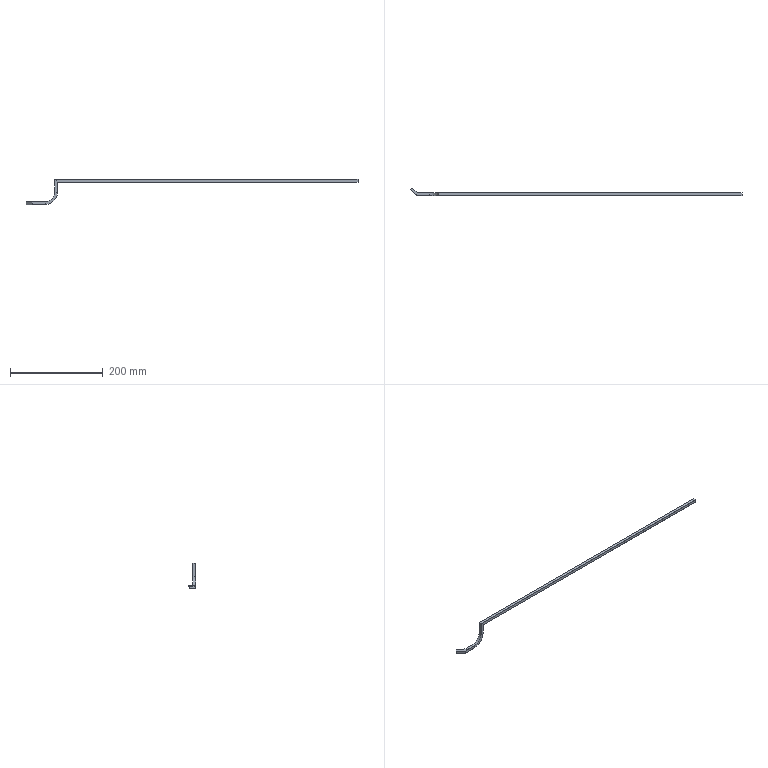Part | STEP file | 1-28.2 | 1 solid | 33 faces | box 716 x 16 x 54 mm | volume 8341 mm3 | plane 30 | cylinder 3 | commonest cylinder face diameters 40 x1 42 x1 52 x1